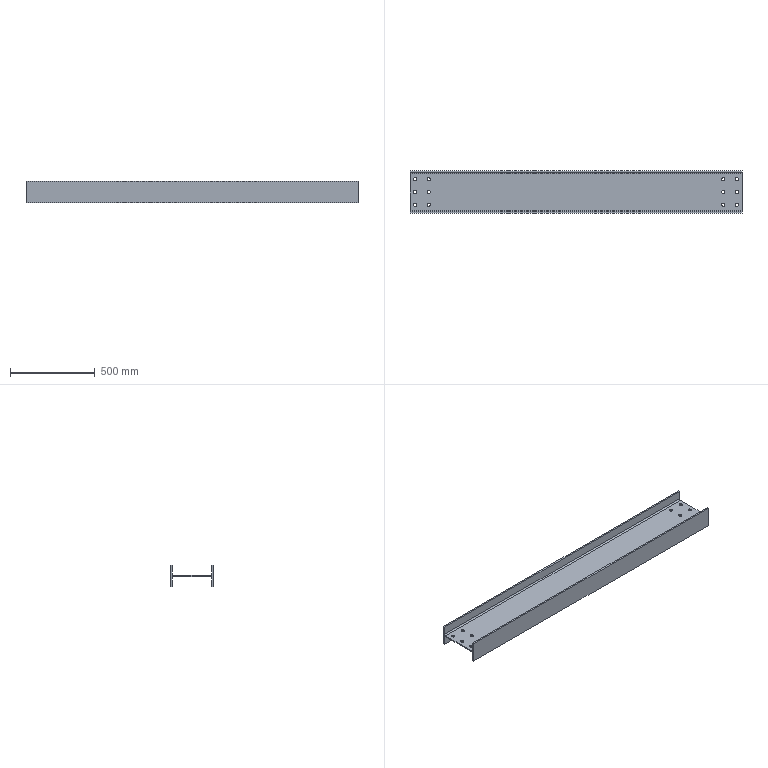Part | STEP file | 粉仓主梁10主体_Default<As Machined> | 1 solid | 42 faces | box 1955 x 250 x 125 mm | volume 7207100 mm3 | cylinder 28 | plane 14 | commonest cylinder face diameters 19 x24 16 x4